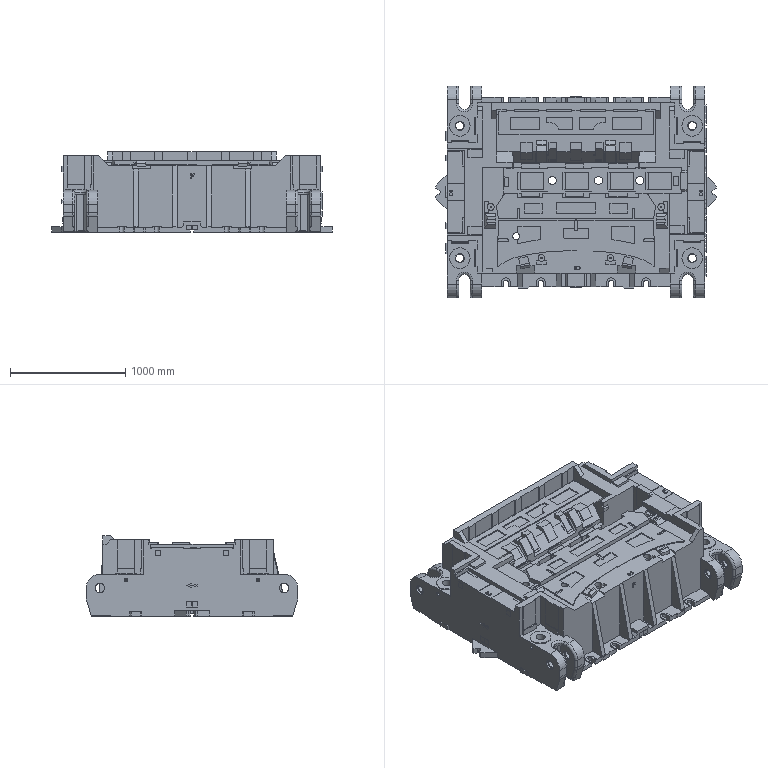Part | NX | features solid 2 | 1 solid | 2337 faces | box 2440 x 1840 x 700 mm | volume 854957554 mm3 | plane 1821 | cylinder 325 | spline 163 | torus 28 | commonest cylinder face diameters 80 x72 83 x48 40 x46 60 x37 10 x27 50 x23